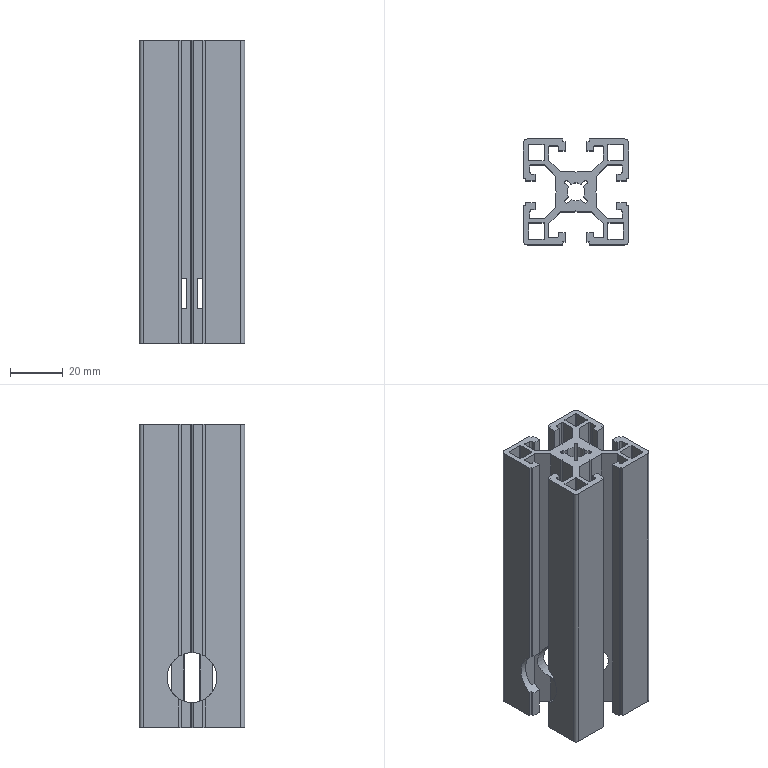Part | NX | features BREP 1 | 1 solid | 218 faces | box 40 x 40 x 115 mm | volume 66336 mm3 | plane 150 | cylinder 68 | commonest cylinder face diameters 0.6 x16 1.5 x12 2 x12 1 x8 6.8 x8 19 x8